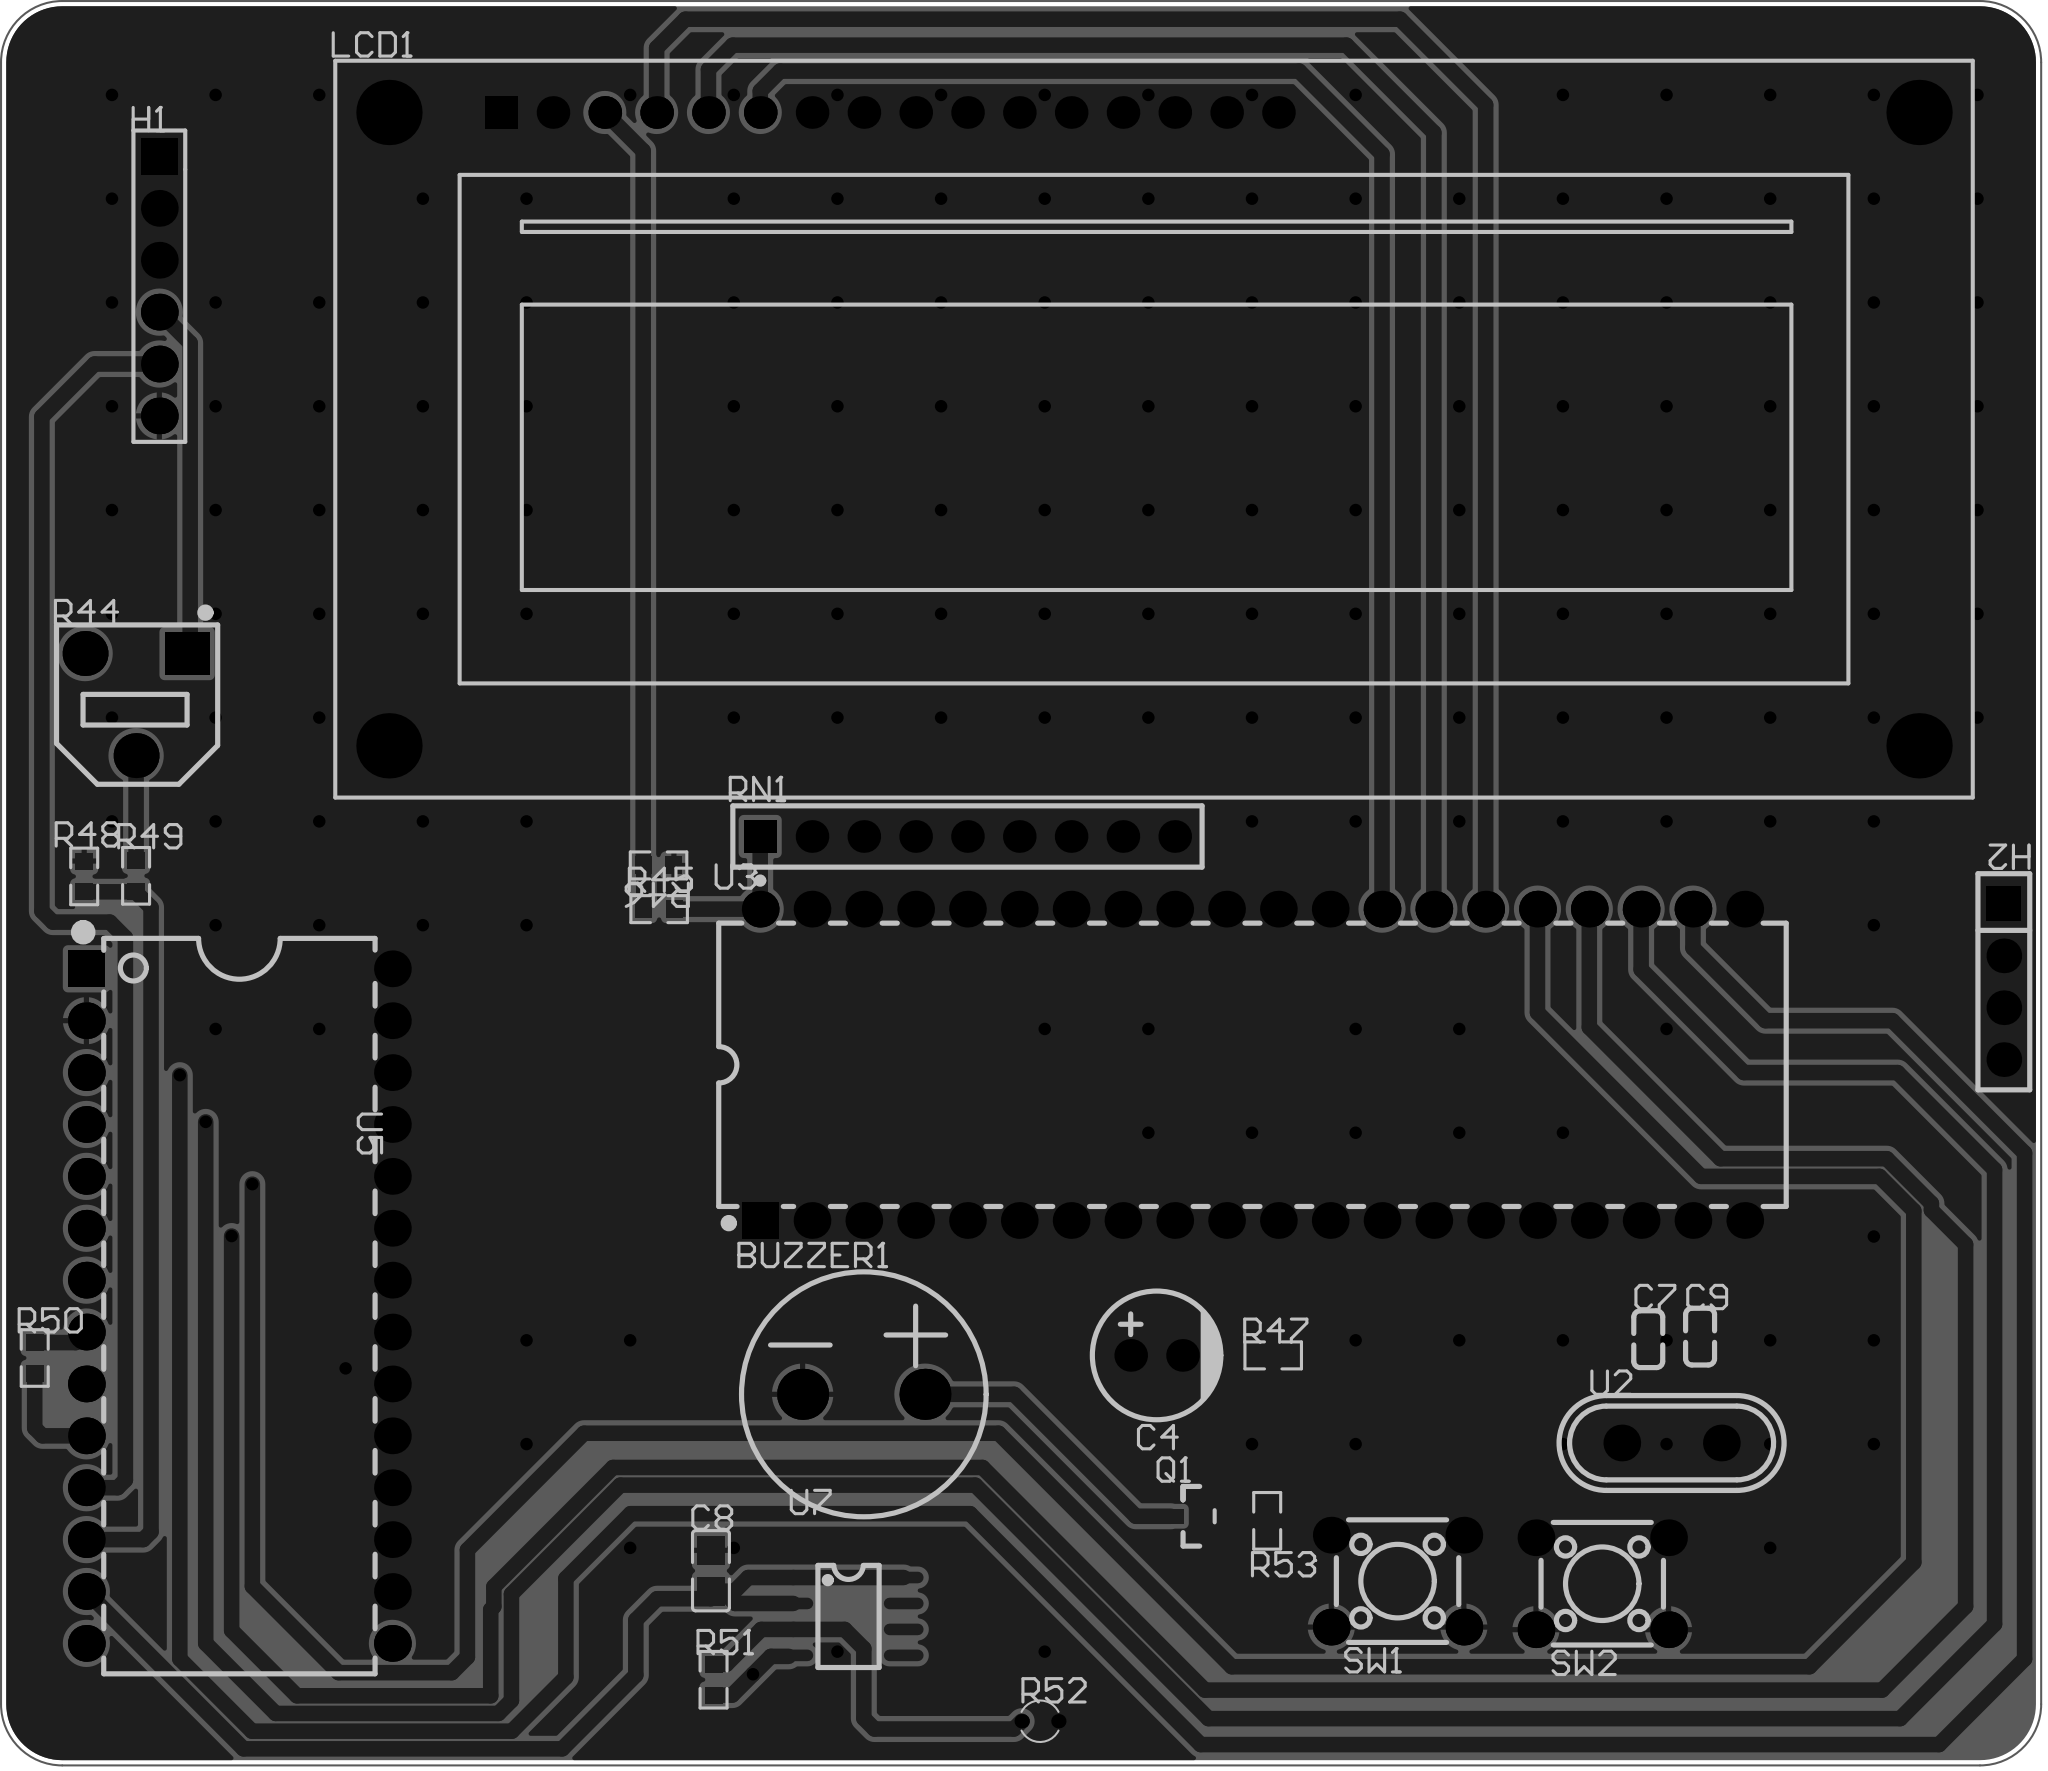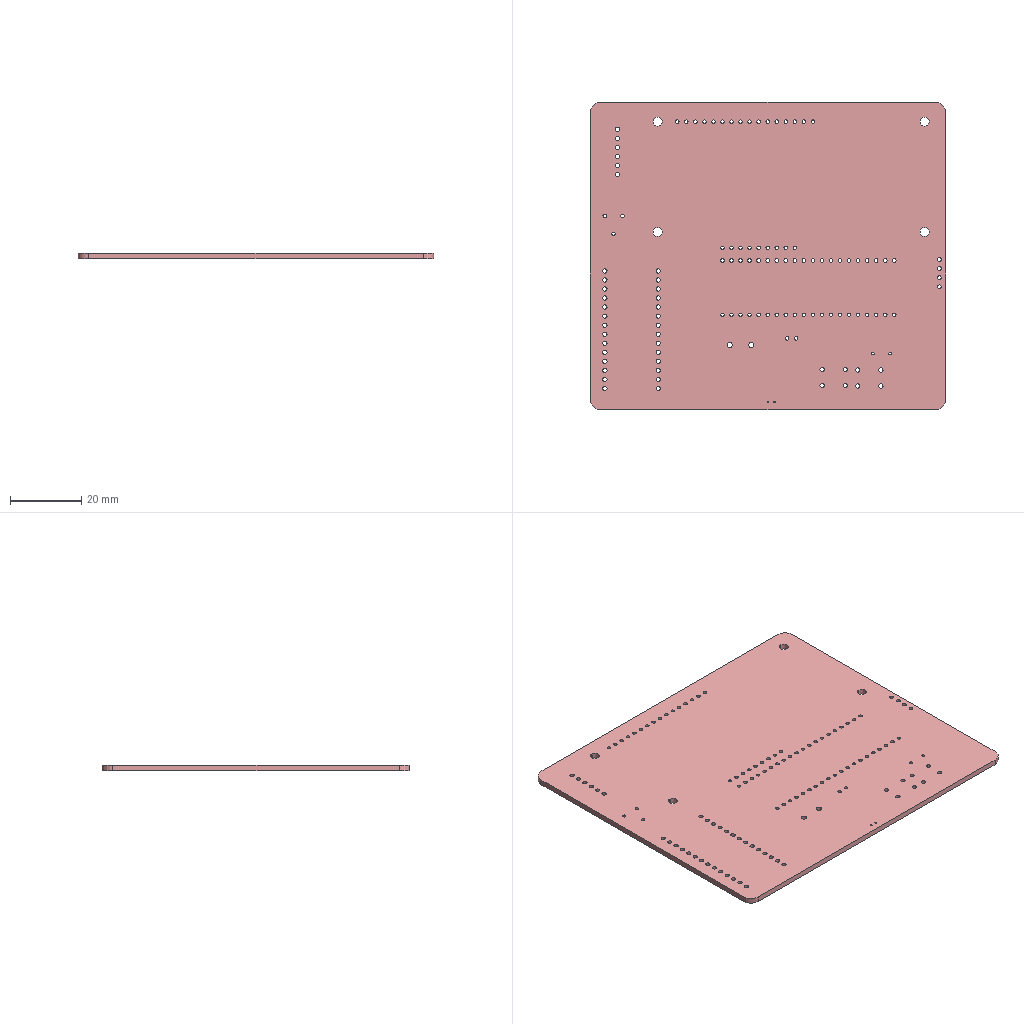Circuit board layout | Altium Designer | box 100 x 86.4 x 1.6 mm
Layer stack:
# Altium Designer layer stack of  (unit mm; dielectric type: 0 none, 1 core, 2 prepreg, 3 surface material)
index,name,kind,layer,copper_thickness_mm,dielectric_type,dielectric_thickness_mm,dielectric_material,dielectric_constant
0,Top Paste Mask Layer,other,,,,,,
1,Top Silkscreen Layer,other,,,,,,
2,Top Solder Mask Layer,dielectric,,,3,0.01,,3.3
3,Top Layer,copper,Top Layer,0.035,,,,
4,Dielectric1,dielectric,,,3,1.51,FR4,4.5
5,Bottom Layer,copper,Bottom Layer,0.035,,,,
6,Bottom Solder Mask Layer,dielectric,,,3,0.01,,3.3
7,Bottom Silkscreen Layer,other,,,,,,
8,Bottom Paste Mask Layer,other,,,,,,
# drill layer pairs: low layer,high layer
drill_pair,Top Layer,Bottom Layer
Part placement:
Designator,Comment,Layer,Footprint,Center-X(mm),Center-Y(mm),Rotation
C4,10uF,TopLayer,CAP-TH_BD6.3-P2.50-D1.0-FD,135.255,100.965,0
BUZZER1,buzzer,TopLayer,BUZ-TH_BD12.0-P6.00-D0.9-RD,120.904,99.06,0
H2,,TopLayer,HDR-TH_4P-P2.54-V-F,176.784,119.253,270
LCD1,LMB162ADC,TopLayer,LCD1602,135.128,146.304,0
Q1,,TopLayer,S8550P_SOT,137.202,93.091,0
R53,2.2K,TopLayer,R0603,140.676,92.868,270
SW1,,TopLayer,SW-TH_4P-L6.0-W6.0-P4.50-LS6.5,147.066,89.916,180
RN1,-,TopLayer,RES-ARRAY-TH_9P-P2.54-D1.0,125.984,126.365,0
U2,12MHz,TopLayer,HC-49US_L11.0-W4.6-P4.88,160.497,96.678,0
U3,STC89C516RD+40I-PDIP40,TopLayer,DIP-40_L52.3-W13.9-P2.54-LS15.2-BL,139.954,115.189,0
SW2,,TopLayer,SW-TH_4P-L6.0-W6.0-P4.50-LS6.5,157.099,89.789,180
C7,22pF,TopLayer,C0603,159.354,101.758,90
C8,100nF,TopLayer,C0805,113.411,90.424,270
C9,22pF,TopLayer,C0603,161.894,101.885,90
R44,10kΩ,TopLayer,RES-ADJ-SMD_RM065-V1,85.233,132.822,180
R45,10K,TopLayer,R0603,110.871,122.809,0
R46,1K,TopLayer,R0603,110.842,124.948,180
R47,10K,TopLayer,R0603,140.97,100.965,180
R48,100K,TopLayer,R0603,82.69,124.41,90
R49,100K,TopLayer,R0603,85.233,124.44,90
R50,50,TopLayer,R0603,80.264,100.838,90
R51,1K,TopLayer,R0603,113.538,85.09,270
U5,AD1674AD,TopLayer,CDIP-28_L35.5-W14.8-P2.54-LS15.3-BL,90.297,103.378,270
H1,,TopLayer,HDR-TH_6P-P2.54-V-M-1,86.373,153.301,270
R52,MF52A502F3435,TopLayer,RES-TH_BD2.0-P1.80-D0.3,129.54,83.058,180
U7,LM358P-CN,TopLayer,SOIC-8_L5.0-W4.0-P1.27-LS6.0-BL,120.154,88.187,270
Pad and via stacks:
# Altium Designer via and pad stacks of  (unit mm). Each distinct definition once, with the count of objects using it.
# via: kind,start_layer,end_layer,hole_mm,diameter_mm,mode(0 simple;1 top-mid-bottom;2 full stack),diameter_per_layer,count,example_net
# pad: kind,layer,hole_mm,hole_type(0 round;1 square;2 slot),plating,top_size,top_shape(1 round;2 rect;3 octagon;9 rounded rect),mid_size,bottom_size,mode,footprint,size_per_layer,count,example
pad,Multi-Layer,1,0,plated,1.6x1.6,1,1.6x1.6,1.6x1.6,0,CAP-TH_BD6.3-P2.50-D1.0-FD,,2,C4.1
pad,Multi-Layer,1.5,0,plated,2.5x2.5,1,2.5x2.5,2.5x2.5,0,BUZ-TH_BD12.0-P6.00-D0.9-RD,,2,BUZZER1.1
pad,Multi-Layer,1.1,0,plated,1.7x1.7,2,1.7x1.7,1.7x1.7,0,HDR-TH_4P-P2.54-V-F,,1,H2.1
pad,Multi-Layer,1.1,0,plated,1.7x1.7,1,1.7x1.7,1.7x1.7,0,HDR-TH_4P-P2.54-V-F,,3,H2.2
pad,Multi-Layer,1,0,plated,1.6x1.6,1,1.6x1.6,1.6x1.6,0,LCD1602,,15,LCD1.16
pad,Multi-Layer,1,0,plated,1.6x1.6,2,1.6x1.6,1.6x1.6,0,LCD1602,,1,LCD1.1
pad,Multi-Layer,2.5,2,plated,3.2x3.2,1,3.2x3.2,3.2x3.2,0,LCD1602,,4,LCD1.0
pad,Multi-Layer,1.2,0,plated,1.8x1.8,1,1.8x1.8,1.8x1.8,0,SW-TH_4P-L6.0-W6.0-P4.50-LS6.5,,8,SW1.1
pad,Multi-Layer,1,0,plated,1.6x1.6,2,1.6x1.6,1.6x1.6,0,RES-ARRAY-TH_9P-P2.54-D1.0,,1,RN1.1
pad,Multi-Layer,1,0,plated,1.6x1.6,1,1.6x1.6,1.6x1.6,0,RES-ARRAY-TH_9P-P2.54-D1.0,,8,RN1.2
pad,Multi-Layer,0.8,0,plated,1.8x1.8,1,1.8x1.8,1.8x1.8,0,HC-49US_L11.0-W4.6-P4.88,,2,U2.1
pad,Multi-Layer,1,0,plated,1.8x1.8,1,1.8x1.8,1.8x1.8,0,DIP-40_L52.3-W13.9-P2.54-LS15.2-BL,,39,U3.19
pad,Multi-Layer,1,0,plated,1.8x1.8,2,1.8x1.8,1.8x1.8,0,DIP-40_L52.3-W13.9-P2.54-LS15.2-BL,,1,U3.1
pad,Multi-Layer,1,0,plated,2.2x2.1,2,2.2x2.1,2.2x2.1,0,RES-ADJ-SMD_RM065-V1,,1,R44.1
pad,Multi-Layer,1,0,plated,2.2x2.2,1,2.2x2.2,2.2x2.2,0,RES-ADJ-SMD_RM065-V1,,2,R44.3
pad,Multi-Layer,1.2,0,plated,1.8x1.8,1,1.8x1.8,1.8x1.8,0,CDIP-28_L35.5-W14.8-P2.54-LS15.3-BL,,27,U5.28
pad,Multi-Layer,1.2,0,plated,1.8x1.8,2,1.8x1.8,1.8x1.8,0,CDIP-28_L35.5-W14.8-P2.54-LS15.3-BL,,1,U5.1
pad,Multi-Layer,1.2,0,plated,1.8x1.8,1,1.8x1.8,1.8x1.8,0,HDR-TH_6P-P2.54-V-M-1,,5,H1.6
pad,Multi-Layer,1.2,0,plated,1.8x1.8,2,1.8x1.8,1.8x1.8,0,HDR-TH_6P-P2.54-V-M-1,,1,H1.1
pad,Multi-Layer,0.5,0,plated,0.7x0.7,1,0.7x0.7,0.7x0.7,0,RES-TH_BD2.0-P1.80-D0.3,,2,R52.1
pad,Top Layer,0,0,plated,0.701x1.25,2,0.701x1.25,0.701x1.25,0,S8550P_SOT,,3,Q1.3
pad,Top Layer,0,0,plated,0.8065x0.864,2,0.8065x0.864,0.8065x0.864,0,R0603,,16,R53.2
pad,Top Layer,0,0,plated,0.8x0.9,2,0.8x0.9,0.8x0.9,0,C0603,,4,C7.2
pad,Top Layer,0,0,plated,1.41x1.35,2,1.41x1.35,1.41x1.35,0,C0805,,2,C8.2
pad,Top Layer,0,0,plated,0.5684x1.95,1,0.5684x1.95,0.5684x1.95,0,SOIC-8_L5.0-W4.0-P1.27-LS6.0-BL,,8,U7.1
via,Top Layer,Bottom Layer,0.3048,0.61,0,,176,$1N22841
Copper pours:
name,layer,net,type(0 solid;1 hatched;2 none)
Top Layer-GND,Top Layer,GND,0
Bottom Layer-GND,Bottom Layer,GND,0